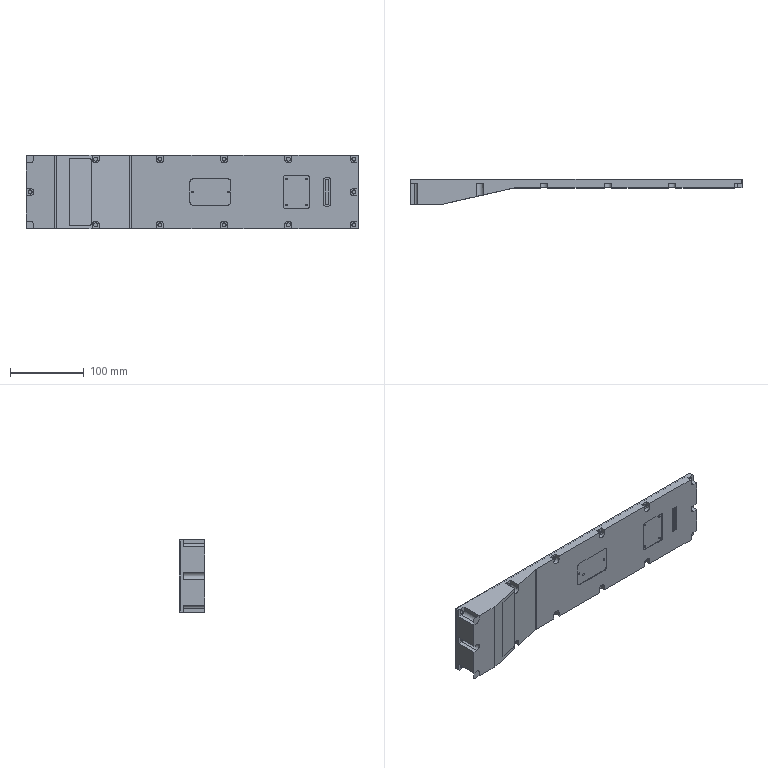NC program | Mastercam | posted with a generic post | part box 450 x 35 x 100 mm
Lines 36 to 1467 of 140701:
(12 FEM |TOOL - 12|DIA. OFF. - 12|LEN. - 12|TOOL DIA. - 12.)
N140 T12 M6
N142 G0 G54 G90 X-233.997 Y-60.496 C0. B0. S7000 M3
N144 G43 H12 Z50.
N146 Z3.
N148 G1 Z-18.575 F600.
N150 X-234.4 Y-59.449 Z-18.7 F4000.
N152 G3 X-235.01 Y-58.51 Z-18.825 I-2.52 J-.971
N154 G1 X-235.205 Y-58.247
N156 X-235.623 Y-57.657
N158 X-235.863 Y-57.277
N160 X-236.1 Y-56.858
N162 X-236.324 Y-56.407
N164 X-236.529 Y-55.928
N166 X-236.708 Y-55.428
N168 X-236.848 Y-54.949
N170 X-236.954 Y-54.508
N172 X-237.033 Y-54.1
N174 X-237.14 Y-53.384
N176 X-237.205 Y-52.737
N178 X-237.245 Y-52.143
N180 X-237.27 Y-51.587
N182 X-237.284 Y-51.058
N184 X-237.293 Y-50.55
N186 X-237.296 Y-50.055
N188 X-237.297 Y-49.569
N190 X-237.296 Y-49.091
N192 X-237.294 Y-48.616
N194 X-237.291 Y-48.145
N196 X-237.287 Y-47.675
N198 X-237.283 Y-47.206
N200 X-237.279 Y-46.738
N202 X-237.275 Y-46.27
N204 X-237.271 Y-45.802
N206 X-237.266 Y-45.334
N208 X-237.262 Y-44.866
N210 X-237.258 Y-44.399
N212 X-237.253 Y-43.931
N214 X-237.249 Y-43.463
N216 X-237.245 Y-42.995
N218 X-237.24 Y-42.526
N220 X-237.236 Y-42.058
N222 X-237.231 Y-41.59
N224 X-237.227 Y-41.121
N226 X-237.222 Y-40.652
N228 X-237.218 Y-40.184
N230 X-237.213 Y-39.715
N232 X-237.209 Y-39.246
N234 X-237.205 Y-38.777
N236 X-237.2 Y-38.307
N238 X-237.196 Y-37.838
N240 X-237.191 Y-37.369
N242 X-237.187 Y-36.899
N244 X-237.182 Y-36.429
N246 X-237.178 Y-35.96
N248 X-237.173 Y-35.49
N250 X-237.169 Y-35.02
N252 X-237.165 Y-34.55
N254 X-237.16 Y-34.08
N256 X-237.156 Y-33.609
N258 X-237.151 Y-33.139
N260 X-237.147 Y-32.669
N262 X-237.142 Y-32.198
N264 X-237.138 Y-31.728
N266 X-237.133 Y-31.257
N268 X-237.129 Y-30.787
N270 X-237.124 Y-30.316
N272 X-237.12 Y-29.845
N274 X-237.116 Y-29.374
N276 X-237.111 Y-28.903
N278 X-237.107 Y-28.432
N280 X-237.102 Y-27.961
N282 X-237.098 Y-27.49
N284 X-237.093 Y-27.018
N286 X-237.089 Y-26.547
N288 X-237.084 Y-26.075
N290 X-237.08 Y-25.604
N292 X-237.075 Y-25.132
N294 X-237.071 Y-24.661
N296 X-237.066 Y-24.189
N298 X-237.062 Y-23.717
N300 X-237.058 Y-23.246
N302 X-237.053 Y-22.774
N304 X-237.049 Y-22.302
N306 X-237.044 Y-21.83
N308 X-237.04 Y-21.358
N310 X-237.035 Y-20.886
N312 X-237.031 Y-20.414
N314 X-237.026 Y-19.941
N316 X-237.022 Y-19.469
N318 X-237.017 Y-18.997
N320 X-237.013 Y-18.524
N322 X-237.008 Y-18.052
N324 X-237.004 Y-17.579
N326 X-236.999 Y-17.107
N328 X-236.995 Y-16.634
N330 X-236.99 Y-16.162
N332 X-236.986 Y-15.689
N334 X-236.982 Y-15.216
N336 X-236.977 Y-14.744
N338 X-236.973 Y-14.271
N340 X-236.968 Y-13.798
N342 X-236.964 Y-13.325
N344 X-236.959 Y-12.852
N346 X-236.955 Y-12.379
N348 X-236.95 Y-11.906
N350 X-236.946 Y-11.433
N352 X-236.941 Y-10.96
N354 X-236.937 Y-10.486
N356 X-236.932 Y-10.013
N358 X-236.928 Y-9.54
N360 X-236.923 Y-9.067
N362 X-236.919 Y-8.593
N364 X-236.914 Y-8.12
N366 X-236.91 Y-7.646
N368 X-236.905 Y-7.173
N370 X-236.901 Y-6.699
N372 X-236.896 Y-6.226
N374 X-236.892 Y-5.752
N376 X-236.887 Y-5.279
N378 X-236.883 Y-4.805
N380 X-236.878 Y-4.331
N382 X-236.874 Y-3.857
N384 X-236.869 Y-3.384
N386 X-236.865 Y-2.91
N388 X-236.861 Y-2.436
N390 X-236.856 Y-1.962
N392 X-236.852 Y-1.488
N394 X-236.847 Y-1.014
N396 X-236.843 Y-.54
N398 X-236.838 Y-.066
N400 X-236.834 Y.408
N402 X-236.829 Y.882
N404 X-236.825 Y1.356
N406 X-236.82 Y1.831
N408 X-236.816 Y2.305
N410 X-236.811 Y2.779
N412 X-236.807 Y3.253
N414 X-236.802 Y3.728
N416 X-236.798 Y4.202
N418 X-236.793 Y4.676
N420 X-236.789 Y5.151
N422 X-236.784 Y5.625
N424 X-236.78 Y6.1
N426 X-236.775 Y6.574
N428 X-236.771 Y7.049
N430 X-236.766 Y7.523
N432 X-236.762 Y7.998
N434 X-236.757 Y8.473
N436 X-236.753 Y8.947
N438 X-236.748 Y9.422
N440 X-236.744 Y9.897
N442 X-236.739 Y10.371
N444 X-236.735 Y10.846
N446 X-236.73 Y11.321
N448 X-236.726 Y11.796
N450 X-236.721 Y12.271
N452 X-236.717 Y12.745
N454 X-236.712 Y13.22
N456 X-236.708 Y13.695
N458 X-236.703 Y14.17
N460 X-236.699 Y14.645
N462 X-236.694 Y15.12
N464 X-236.69 Y15.595
N466 X-236.685 Y16.07
N468 X-236.681 Y16.546
N470 X-236.676 Y17.021
N472 X-236.672 Y17.496
N474 X-236.667 Y17.971
N476 X-236.663 Y18.446
N478 X-236.658 Y18.921
N480 X-236.654 Y19.397
N482 X-236.649 Y19.872
N484 X-236.645 Y20.347
N486 X-236.64 Y20.823
N488 X-236.636 Y21.298
N490 X-236.631 Y21.773
N492 X-236.627 Y22.249
N494 X-236.622 Y22.724
N496 X-236.618 Y23.2
N498 X-236.613 Y23.675
N500 X-236.609 Y24.15
N502 X-236.604 Y24.626
N504 X-236.6 Y25.102
N506 X-236.595 Y25.577
N508 X-236.591 Y26.053
N510 X-236.586 Y26.528
N512 X-236.582 Y27.004
N514 X-236.577 Y27.48
N516 X-236.573 Y27.955
N518 X-236.568 Y28.431
N520 X-236.564 Y28.907
N522 X-236.559 Y29.382
N524 X-236.555 Y29.858
N526 X-236.55 Y30.334
N528 X-236.546 Y30.81
N530 X-236.541 Y31.286
N532 X-236.537 Y31.761
N534 X-236.532 Y32.237
N536 X-236.528 Y32.714
N538 X-236.524 Y33.191
N540 X-236.521 Y33.669
N542 X-236.518 Y34.148
N544 X-236.516 Y34.627
N546 X-236.513 Y35.107
N548 X-236.512 Y35.587
N550 X-236.51 Y36.068
N552 X-236.509 Y36.549
N554 X-236.508 Y37.03
N556 X-236.507 Y37.511
N558 X-236.506 Y37.993
N560 X-236.505 Y38.475
N562 X-236.504 Y38.957
N564 Y39.439
N566 X-236.503 Y39.921
N568 Y40.403
N570 X-236.502 Y40.885
N572 Y41.368
N574 Y41.85
N576 Y42.332
N578 X-236.501 Y42.815
N580 Y43.298
N582 Y43.78
N584 Y44.263
N586 Y44.745
N588 Y45.228
N590 Y45.711
N592 X-236.5 Y46.193
N594 Y46.676
N596 Y47.159
N598 Y47.642
N600 Y48.124
N602 Y48.607
N604 Y49.09
N606 X-236.499 Y49.611
N608 X-236.485 Y50.23
N610 X-236.44 Y50.918
N612 X-236.401 Y51.288
N614 X-236.347 Y51.666
N616 X-236.277 Y52.051
N618 X-236.19 Y52.44
N620 X-236.085 Y52.831
N622 X-235.96 Y53.221
N624 X-235.816 Y53.607
N626 X-235.651 Y53.989
N628 X-235.466 Y54.362
N630 X-235.26 Y54.727
N632 X-235.034 Y55.079
N634 X-234.788 Y55.418
N636 X-234.524 Y55.743
N638 X-234.245 Y56.051
N640 X-233.952 Y56.343
N642 X-233.649 Y56.618
N644 X-233.337 Y56.875
N646 X-233.018 Y57.116
N648 X-232.694 Y57.34
N650 X-232.366 Y57.548
N652 X-232.036 Y57.741
N654 X-231.705 Y57.919
N656 X-231.056 Y58.23
N658 X-230.41 Y58.496
N660 X-229.773 Y58.721
N662 X-229.146 Y58.912
N664 X-228.53 Y59.074
N666 X-227.927 Y59.211
N668 X-227.336 Y59.327
N670 X-226.756 Y59.425
N672 X-226.187 Y59.508
N674 X-225.627 Y59.579
N676 X-225.077 Y59.639
N678 X-224.535 Y59.691
N680 X-224.001 Y59.734
N682 X-223.473 Y59.772
N684 X-222.95 Y59.804
N686 X-222.433 Y59.831
N688 X-221.92 Y59.855
N690 X-221.411 Y59.875
N692 X-220.906 Y59.892
N694 X-220.403 Y59.907
N696 X-219.903 Y59.92
N698 X-219.406 Y59.931
N700 X-218.91 Y59.94
N702 X-218.416 Y59.949
N704 X-217.924 Y59.956
N706 X-217.433 Y59.962
N708 X-216.942 Y59.967
N710 X-216.453 Y59.971
N712 X-215.965 Y59.975
N714 X-215.478 Y59.979
N716 X-214.991 Y59.982
N718 X-214.505 Y59.984
N720 X-214.019 Y59.986
N722 X-213.533 Y59.988
N724 X-213.048 Y59.99
N726 X-212.563 Y59.991
N728 X-212.079 Y59.992
N730 X-211.595 Y59.993
N732 X-211.111 Y59.994
N734 X-210.627 Y59.995
N736 X-210.143 Y59.996
N738 X-209.659
N740 X-209.176 Y59.997
N742 X-208.692
N744 X-208.209 Y59.998
N746 X-207.726
N748 X-207.243
N750 X-206.759
N752 X-206.276 Y59.999
N754 X-205.793
N756 X-205.31
N758 X-204.827
N760 X-204.344
N762 X-203.861
N764 X-203.378
N766 X-202.895 Y60.
N768 X-202.412
N770 X-201.93
N772 X-201.447
N774 X-200.964
N776 X-200.481
N778 X-199.998
N780 X-199.515
N782 X-199.032
N784 X-198.55
N786 X-198.067
N788 X-197.584
N790 X-197.101
N792 X-196.618
N794 X-196.135
N796 X-195.653
N798 X-195.17
N800 X-194.687
N802 X-194.204
N804 X-193.721
N806 X-193.238
N808 X-192.756
N810 X-192.273
N812 X-191.79
N814 X-191.307
N816 X-190.824
N818 X-190.342
N820 X-189.859
N822 X-189.376
N824 X-188.893
N826 X-188.41
N828 X-187.927
N830 X-187.445
N832 X-186.962
N834 X-186.479
N836 X-185.996
N838 X-185.513
N840 X-185.031
N842 X-184.548
N844 X-184.065
N846 X-183.582
N848 X-183.099
N850 X-182.616
N852 X-182.134
N854 X-181.651
N856 X-181.168
N858 X-180.685
N860 X-180.202
N862 X-179.72
N864 X-179.237
N866 X-178.754
N868 X-178.271
N870 X-177.788
N872 X-177.306
N874 X-176.823
N876 X-176.34
N878 X-175.857
N880 X-175.374
N882 X-174.891
N884 X-174.409
N886 X-173.926
N888 X-173.443
N890 X-172.96
N892 X-172.477
N894 X-171.995
N896 X-171.512
N898 X-171.029
N900 X-170.546
N902 X-170.063
N904 X-169.581
N906 X-169.098
N908 X-168.615
N910 X-168.132
N912 X-167.649
N914 X-167.166
N916 X-166.684
N918 X-166.201
N920 X-165.718
N922 X-165.235
N924 X-164.752
N926 X-164.27
N928 X-163.787
N930 X-163.304
N932 X-162.821
N934 X-162.338
N936 X-161.856
N938 X-161.373
N940 X-160.89
N942 X-160.407
N944 X-159.924
N946 X-159.441
N948 X-158.959
N950 X-158.476
N952 X-157.993
N954 X-157.51
N956 X-157.027
N958 X-156.545
N960 X-156.062
N962 X-155.579
N964 X-155.096
N966 X-154.613
N968 X-154.131
N970 X-153.648
N972 X-153.165
N974 X-152.682
N976 X-152.199
N978 X-151.716
N980 X-151.234
N982 X-150.751
N984 X-150.268
N986 X-149.785
N988 X-149.302
N990 X-148.82
N992 X-148.337
N994 X-147.854
N996 X-147.371
N998 X-146.888
N1000 X-146.406
N1002 X-145.923
N1004 X-145.44
N1006 X-144.957
N1008 X-144.474
N1010 X-143.991
N1012 X-143.509
N1014 X-143.026
N1016 X-142.543
N1018 X-142.06
N1020 X-141.577
N1022 X-141.095
N1024 X-140.612
N1026 X-140.129
N1028 X-139.646
N1030 X-139.163
N1032 X-138.681
N1034 X-138.198
N1036 X-137.715
N1038 X-137.232
N1040 X-136.749
N1042 X-136.266
N1044 X-135.784
N1046 X-135.301
N1048 X-134.818
N1050 X-134.335
N1052 X-133.852
N1054 X-133.37
N1056 X-132.887
N1058 X-132.404
N1060 X-131.921
N1062 X-131.438
N1064 X-130.956
N1066 X-130.473
N1068 X-129.99
N1070 X-129.507
N1072 X-129.024
N1074 X-128.542
N1076 X-128.059
N1078 X-127.576
N1080 X-127.093
N1082 X-126.61
N1084 X-126.127
N1086 X-125.645
N1088 X-125.162
N1090 X-124.679
N1092 X-124.196
N1094 X-123.713
N1096 X-123.231
N1098 X-122.748
N1100 X-122.265
N1102 X-121.782
N1104 X-121.299
N1106 X-120.817
N1108 X-120.334
N1110 X-119.851
N1112 X-119.368
N1114 X-118.885
N1116 X-118.402
N1118 X-117.92
N1120 X-117.437
N1122 X-116.954
N1124 X-116.471
N1126 X-115.988
N1128 X-115.506
N1130 X-115.023
N1132 X-114.54
N1134 X-114.057
N1136 X-113.574
N1138 X-113.092
N1140 X-112.609
N1142 X-112.126
N1144 X-111.643
N1146 X-111.16
N1148 X-110.677
N1150 X-110.195
N1152 X-109.712
N1154 X-109.229
N1156 X-108.746
N1158 X-108.263
N1160 X-107.781
N1162 X-107.298
N1164 X-106.815
N1166 X-106.332
N1168 X-105.849
N1170 X-105.367
N1172 X-104.884
N1174 X-104.401
N1176 X-103.918
N1178 X-103.435
N1180 X-102.952
N1182 X-102.47
N1184 X-101.987
N1186 X-101.504
N1188 X-101.021
N1190 X-100.538
N1192 X-100.056
N1194 X-99.573
N1196 X-99.09
N1198 X-98.607
N1200 X-98.124
N1202 X-97.642
N1204 X-97.159
N1206 X-96.676
N1208 X-96.193
N1210 X-95.71
N1212 X-95.227
N1214 X-94.745
N1216 X-94.262
N1218 X-93.779
N1220 X-93.296
N1222 X-92.813
N1224 X-92.331
N1226 X-91.848
N1228 X-91.365
N1230 X-90.882
N1232 X-90.399
N1234 X-89.917
N1236 X-89.434
N1238 X-88.951
N1240 X-88.468
N1242 X-87.985
N1244 X-87.502
N1246 X-87.02
N1248 X-86.537
N1250 X-86.054
N1252 X-85.571
N1254 X-85.088
N1256 X-84.606
N1258 X-84.123
N1260 X-83.64
N1262 X-83.157
N1264 X-82.674
N1266 X-82.192
N1268 X-81.709
N1270 X-81.226
N1272 X-80.743
N1274 X-80.26
N1276 X-79.777
N1278 X-79.295
N1280 X-78.812
N1282 X-78.329
N1284 X-77.846
N1286 X-77.363
N1288 X-76.881
N1290 X-76.398
N1292 X-75.915
N1294 X-75.432
N1296 X-74.949
N1298 X-74.467
N1300 X-73.984
N1302 X-73.501
N1304 X-73.018
N1306 X-72.535
N1308 X-72.052
N1310 X-71.57
N1312 X-71.087
N1314 X-70.604
N1316 X-70.121
N1318 X-69.638
N1320 X-69.156
N1322 X-68.673
N1324 X-68.19
N1326 X-67.707
N1328 X-67.224
N1330 X-66.742
N1332 X-66.259
N1334 X-65.776
N1336 X-65.293
N1338 X-64.81
N1340 X-64.327
N1342 X-63.845
N1344 X-63.362
N1346 X-62.879
N1348 X-62.396
N1350 X-61.913
N1352 X-61.431
N1354 X-60.948
N1356 X-60.465
N1358 X-59.982
N1360 X-59.499
N1362 X-59.017
N1364 X-58.534
N1366 X-58.051
N1368 X-57.568
N1370 X-57.085
N1372 X-56.602
N1374 X-56.12
N1376 X-55.637
N1378 X-55.154
N1380 X-54.671
N1382 X-54.188
N1384 X-53.706
N1386 X-53.223
N1388 X-52.74
N1390 X-52.257
N1392 X-51.774
N1394 X-51.292
N1396 X-50.809
N1398 X-50.326
N1400 X-49.843
N1402 X-49.36
N1404 X-48.877
N1406 X-48.395
N1408 X-47.912
N1410 X-47.429
N1412 X-46.946
N1414 X-46.463
N1416 X-45.981
N1418 X-45.498
N1420 X-45.015
N1422 X-44.532
N1424 X-44.049
N1426 X-43.567
N1428 X-43.084
N1430 X-42.601
N1432 X-42.118
N1434 X-41.635
N1436 X-41.152
N1438 X-40.67
N1440 X-40.187
N1442 X-39.704
N1444 X-39.221
N1446 X-38.738
N1448 X-38.256
N1450 X-37.773
N1452 X-37.29
N1454 X-36.807
N1456 X-36.324
N1458 X-35.842
N1460 X-35.359
N1462 X-34.876
N1464 X-34.393
N1466 X-33.91
N1468 X-33.427
N1470 X-32.945
N1472 X-32.462
N1474 X-31.979
N1476 X-31.496
N1478 X-31.013
N1480 X-30.531
N1482 X-30.048
N1484 X-29.565
N1486 X-29.082
N1488 X-28.599
N1490 X-28.117
N1492 X-27.634
N1494 X-27.151
N1496 X-26.668
N1498 X-26.185
N1500 X-25.702
N1502 X-25.22
N1504 X-24.737
N1506 X-24.254
N1508 X-23.771
N1510 X-23.288
N1512 X-22.806
N1514 X-22.323
N1516 X-21.84
N1518 X-21.357
N1520 X-20.874
N1522 X-20.392
N1524 X-19.909
N1526 X-19.426
N1528 X-18.943
N1530 X-18.46
N1532 X-17.977
N1534 X-17.495
N1536 X-17.012
N1538 X-16.529
N1540 X-16.046
N1542 X-15.563
N1544 X-15.081
N1546 X-14.598
N1548 X-14.115
N1550 X-13.632
N1552 X-13.149
N1554 X-12.667
N1556 X-12.184
N1558 X-11.701
N1560 X-11.218
N1562 X-10.735
N1564 X-10.252
N1566 X-9.77
N1568 X-9.287
N1570 X-8.804
N1572 X-8.321
N1574 X-7.838
N1576 X-7.356
N1578 X-6.873
N1580 X-6.39
N1582 X-5.907
N1584 X-5.424
N1586 X-4.942
N1588 X-4.459
N1590 X-3.976
N1592 X-3.493
N1594 X-3.01
N1596 X-2.527
N1598 X-2.045
N1600 X-1.562
N1602 X-1.079
N1604 X-.596
N1606 X-.113
N1608 X.369
N1610 X.852
N1612 X1.335
N1614 X1.818
N1616 X2.301
N1618 X2.783
N1620 X3.266
N1622 X3.749
N1624 X4.232
N1626 X4.715
N1628 X5.198
N1630 X5.68
N1632 X6.163
N1634 X6.646
N1636 X7.129
N1638 X7.612
N1640 X8.094
N1642 X8.577
N1644 X9.06
N1646 X9.543
N1648 X10.026
N1650 X10.508
N1652 X10.991
N1654 X11.474
N1656 X11.957
N1658 X12.44
N1660 X12.923
N1662 X13.405
N1664 X13.888
N1666 X14.371
N1668 X14.854
N1670 X15.337
N1672 X15.819
N1674 X16.302
N1676 X16.785
N1678 X17.268
N1680 X17.751
N1682 X18.233
N1684 X18.716
N1686 X19.199
N1688 X19.682
N1690 X20.165
N1692 X20.648
N1694 X21.13
N1696 X21.613
N1698 X22.096
N1700 X22.579
N1702 X23.062
N1704 X23.544
N1706 X24.027
N1708 X24.51
N1710 X24.993
N1712 X25.476
N1714 X25.958
N1716 X26.441
N1718 X26.924
N1720 X27.407
N1722 X27.89
N1724 X28.373
N1726 X28.855
N1728 X29.338
N1730 X29.821
N1732 X30.304
N1734 X30.787
N1736 X31.269
N1738 X31.752
N1740 X32.235
N1742 X32.718
N1744 X33.201
N1746 X33.683
N1748 X34.166
N1750 X34.649
N1752 X35.132
N1754 X35.615
N1756 X36.098
N1758 X36.58
N1760 X37.063
N1762 X37.546
N1764 X38.029
N1766 X38.512
N1768 X38.994
N1770 X39.477
N1772 X39.96
N1774 X40.443
N1776 X40.926
N1778 X41.408
N1780 X41.891
N1782 X42.374
N1784 X42.857
N1786 X43.34
N1788 X43.823
N1790 X44.305
N1792 X44.788
N1794 X45.271
N1796 X45.754
N1798 X46.237
N1800 X46.719
N1802 X47.202
N1804 X47.685
N1806 X48.168
N1808 X48.651
N1810 X49.133
N1812 X49.616
N1814 X50.099
N1816 X50.582
N1818 X51.065
N1820 X51.548
N1822 X52.03
N1824 X52.513
N1826 X52.996
N1828 X53.479
N1830 X53.962
N1832 X54.444
N1834 X54.927
N1836 X55.41
N1838 X55.893
N1840 X56.376
N1842 X56.858
N1844 X57.341
N1846 X57.824
N1848 X58.307
N1850 X58.79
N1852 X59.273
N1854 X59.755
N1856 X60.238
N1858 X60.721
N1860 X61.204
N1862 X61.687
N1864 X62.169
N1866 X62.652
N1868 X63.135
N1870 X63.618
N1872 X64.101
N1874 X64.583
N1876 X65.066
N1878 X65.549
N1880 X66.032
N1882 X66.515
N1884 X66.998
N1886 X67.48
N1888 X67.963
N1890 X68.446
N1892 X68.929
N1894 X69.412
N1896 X69.894
N1898 X70.377
N1900 X70.86
N1902 X71.343
N1904 X71.826
N1906 X72.308
N1908 X72.791
N1910 X73.274
N1912 X73.757
N1914 X74.24
N1916 X74.723
N1918 X75.205
N1920 X75.688
N1922 X76.171
N1924 X76.654
N1926 X77.137
N1928 X77.619
N1930 X78.102
N1932 X78.585
N1934 X79.068
N1936 X79.551
N1938 X80.033
N1940 X80.516
N1942 X80.999
N1944 X81.482
N1946 X81.965
N1948 X82.448
N1950 X82.93
N1952 X83.413
N1954 X83.896
N1956 X84.379
N1958 X84.862
N1960 X85.344
N1962 X85.827
N1964 X86.31
N1966 X86.793
N1968 X87.276
N1970 X87.758
N1972 X88.241
N1974 X88.724
N1976 X89.207
N1978 X89.69
N1980 X90.173
N1982 X90.655
N1984 X91.138
N1986 X91.621
N1988 X92.104
N1990 X92.587
N1992 X93.069
N1994 X93.552
N1996 X94.035
N1998 X94.518
N2000 X95.001
N2002 X95.483
N2004 X95.966
N2006 X96.449
N2008 X96.932
N2010 X97.415
N2012 X97.898
N2014 X98.38
N2016 X98.863
N2018 X99.346
N2020 X99.829
N2022 X100.312
N2024 X100.794
N2026 X101.277
N2028 X101.76
N2030 X102.243
N2032 X102.726
N2034 X103.208
N2036 X103.691
N2038 X104.174
N2040 X104.657
N2042 X105.14
N2044 X105.623
N2046 X106.105
N2048 X106.588
N2050 X107.071
N2052 X107.554
N2054 X108.037
N2056 X108.519
N2058 X109.002
N2060 X109.485
N2062 X109.968
N2064 X110.451
N2066 X110.933
N2068 X111.416
N2070 X111.899
N2072 X112.382
N2074 X112.865
N2076 X113.348
N2078 X113.83
N2080 X114.313
N2082 X114.796
N2084 X115.279
N2086 X115.762
N2088 X116.244
N2090 X116.727
N2092 X117.21
N2094 X117.693
N2096 X118.176
N2098 X118.658
N2100 X119.141
N2102 X119.624
N2104 X120.107
N2106 X120.59
N2108 X121.073
N2110 X121.555
N2112 X122.038
N2114 X122.521
N2116 X123.004
N2118 X123.487
N2120 X123.969
N2122 X124.452
N2124 X124.935
N2126 X125.418
N2128 X125.901
N2130 X126.383
N2132 X126.866
N2134 X127.349
N2136 X127.832
N2138 X128.315
N2140 X128.798
N2142 X129.28
N2144 X129.763
N2146 X130.246
N2148 X130.729
N2150 X131.212
N2152 X131.694
N2154 X132.177
N2156 X132.66
N2158 X133.143
N2160 X133.626
N2162 X134.108
N2164 X134.591
N2166 X135.074
N2168 X135.557
N2170 X136.04
N2172 X136.523
N2174 X137.005
N2176 X137.488
N2178 X137.971
N2180 X138.454
N2182 X138.937
N2184 X139.419
N2186 X139.902
N2188 X140.385
N2190 X140.868
N2192 X141.351
N2194 X141.833
N2196 X142.316
N2198 X142.799
N2200 X143.282
N2202 X143.765
N2204 X144.247
N2206 X144.73
N2208 X145.213
N2210 X145.696
N2212 X146.179
N2214 X146.662
N2216 X147.144
N2218 X147.627
N2220 X148.11
N2222 X148.593
N2224 X149.076
N2226 X149.558
N2228 X150.041
N2230 X150.524
N2232 X151.007
N2234 X151.49
N2236 X151.972
N2238 X152.455
N2240 X152.938
N2242 X153.421
N2244 X153.904
N2246 X154.387
N2248 X154.869
N2250 X155.352
N2252 X155.835
N2254 X156.318
N2256 X156.801
N2258 X157.283
N2260 X157.766
N2262 X158.249
N2264 X158.732
N2266 X159.215
N2268 X159.697
N2270 X160.18
N2272 X160.663
N2274 X161.146
N2276 X161.629
N2278 X162.112
N2280 X162.594
N2282 X163.077
N2284 X163.56
N2286 X164.043
N2288 X164.526
N2290 X165.008
N2292 X165.491
N2294 X165.974
N2296 X166.457
N2298 X166.94
N2300 X167.422
N2302 X167.905
N2304 X168.388
N2306 X168.871
N2308 X169.354
N2310 X169.837
N2312 X170.319
N2314 X170.802
N2316 X171.285
N2318 X171.768
N2320 X172.251
N2322 X172.733
N2324 X173.216
N2326 X173.699
N2328 X174.182
N2330 X174.665
N2332 X175.147
N2334 X175.63
N2336 X176.113
N2338 X176.596
N2340 X177.079
N2342 X177.562
N2344 X178.044
N2346 X178.527
N2348 X179.01
N2350 X179.493
N2352 X179.976
N2354 X180.458
N2356 X180.941
N2358 X181.424
N2360 X181.907
N2362 X182.39
N2364 X182.872
N2366 X183.355
N2368 X183.838
N2370 X184.321
N2372 X184.804
N2374 X185.287
N2376 X185.769
N2378 X186.252
N2380 X186.735
N2382 X187.218
N2384 X187.701
N2386 X188.183
N2388 X188.666
N2390 X189.149
N2392 X189.632
N2394 X190.115
N2396 X190.597
N2398 X191.08
N2400 X191.563
N2402 X192.046
N2404 X192.529
N2406 X193.012
N2408 X193.494
N2410 X193.977
N2412 X194.46
N2414 X194.943
N2416 X195.426
N2418 X195.908
N2420 X196.391
N2422 X196.874
N2424 X197.357
N2426 X197.84
N2428 X198.322
N2430 X198.805
N2432 X199.288
N2434 X199.771
N2436 X200.254
N2438 X200.737
N2440 X201.219
N2442 X201.702
N2444 X202.185
N2446 X202.668
N2448 X203.151
N2450 X203.633
N2452 X204.116
N2454 X204.599
N2456 X205.082
N2458 X205.565
N2460 X206.047
N2462 X206.53
N2464 X207.013
N2466 X207.496
N2468 X207.979
N2470 X208.462
N2472 X208.944
N2474 X209.427
N2476 X209.91
N2478 X210.393
N2480 X210.876
N2482 X211.358
N2484 X211.841
N2486 X212.324
N2488 X212.807
N2490 X213.29
N2492 X213.772
N2494 X214.255
N2496 X214.738
N2498 X215.221
N2500 X215.704
N2502 X216.187
N2504 X216.669
N2506 X217.152
N2508 X217.635
N2510 X218.118
N2512 X218.601
N2514 X219.083
N2516 X219.566
N2518 X220.049
N2520 X220.532
N2522 X221.015
N2524 X221.497
N2526 X221.98
N2528 X222.463
N2530 X222.946
N2532 X223.429
N2534 X223.912
N2536 X224.394
N2538 X224.877
N2540 X225.36
N2542 X225.849
N2544 X226.425 Y59.994
N2546 X227.084 Y59.966
N2548 X227.798 Y59.899
N2550 X228.177 Y59.845
N2552 X228.562 Y59.775
N2554 X228.952 Y59.687
N2556 X229.342 Y59.582
N2558 X229.732 Y59.457
N2560 X230.119 Y59.312
N2562 X230.5 Y59.146
N2564 X230.873 Y58.96
N2566 X231.237 Y58.754
N2568 X231.589 Y58.527
N2570 X231.928 Y58.28
N2572 X232.252 Y58.016
N2574 X232.56 Y57.736
N2576 X232.851 Y57.444
N2578 X233.125 Y57.14
N2580 X233.382 Y56.828
N2582 X233.622 Y56.509
N2584 X233.846 Y56.184
N2586 X234.054 Y55.856
N2588 X234.246 Y55.526
N2590 X234.424 Y55.195
N2592 X234.734 Y54.546
N2594 X234.999 Y53.901
N2596 X235.224 Y53.264
N2598 X235.415 Y52.637
N2600 X235.576 Y52.021
N2602 X235.712 Y51.418
N2604 X235.828 Y50.827
N2606 X235.926 Y50.247
N2608 X236.009 Y49.678
N2610 X236.08 Y49.119
N2612 X236.14 Y48.569
N2614 X236.191 Y48.027
N2616 X236.235 Y47.493
N2618 X236.272 Y46.965
N2620 X236.304 Y46.443
N2622 X236.332 Y45.925
N2624 X236.355 Y45.413
N2626 X236.375 Y44.904
N2628 X236.392 Y44.398
N2630 X236.407 Y43.896
N2632 X236.42 Y43.396
N2634 X236.431 Y42.898
N2636 X236.441 Y42.403
N2638 X236.449 Y41.909
N2640 X236.456 Y41.416
N2642 X236.462 Y40.925
N2644 X236.467 Y40.435
N2646 X236.471 Y39.946
N2648 X236.475 Y39.458
N2650 X236.479 Y38.971
N2652 X236.482 Y38.484
N2654 X236.484 Y37.997
N2656 X236.486 Y37.512
N2658 X236.488 Y37.026
N2660 X236.49 Y36.541
N2662 X236.491 Y36.056
N2664 X236.492 Y35.572
N2666 X236.493 Y35.088
N2668 X236.494 Y34.603
N2670 X236.495 Y34.12
N2672 X236.496 Y33.636
N2674 Y33.152
N2676 X236.497 Y32.669
N2678 Y32.185
N2680 X236.498 Y31.702
N2682 Y31.219
N2684 Y30.735
N2686 Y30.252
N2688 X236.499 Y29.769
N2690 Y29.286
N2692 Y28.803
N2694 Y28.32
N2696 Y27.837
N2698 Y27.354
N2700 Y26.871
N2702 X236.5 Y26.388
N2704 Y25.905
N2706 Y25.422
N2708 Y24.94
N2710 Y24.457
N2712 Y23.974
N2714 Y23.491
N2716 Y23.008
N2718 Y22.525
N2720 Y22.042
N2722 Y21.56
N2724 Y21.077
N2726 Y20.594
N2728 Y20.111
N2730 Y19.628
N2732 Y19.145
N2734 Y18.663
N2736 Y18.18
N2738 Y17.697
N2740 Y17.214
N2742 Y16.731
N2744 Y16.249
N2746 Y15.766
N2748 Y15.283
N2750 Y14.8
N2752 Y14.317
N2754 Y13.834
N2756 Y13.352
N2758 Y12.869
N2760 Y12.386
N2762 Y11.903
N2764 Y11.42
N2766 Y10.938
N2768 Y10.455
N2770 Y9.972
N2772 Y9.489
N2774 Y9.006
N2776 Y8.523
N2778 Y8.041
N2780 Y7.558
N2782 Y7.075
N2784 Y6.592
N2786 Y6.109
N2788 Y5.627
N2790 Y5.144
N2792 Y4.661
N2794 Y4.178
N2796 Y3.695
N2798 Y3.213
N2800 Y2.73
N2802 Y2.247
N2804 Y1.764
N2806 Y1.281
N2808 Y.798
N2810 Y.316
N2812 Y-.167
N2814 Y-.65
N2816 Y-1.133
N2818 Y-1.616
N2820 Y-2.098
N2822 Y-2.581
N2824 Y-3.064
N2826 Y-3.547
N2828 Y-4.03
N2830 Y-4.512
N2832 Y-4.995
N2834 Y-5.478
N2836 Y-5.961
N2838 Y-6.444
N2840 Y-6.927
N2842 Y-7.409
N2844 Y-7.892
N2846 Y-8.375
N2848 Y-8.858
N2850 Y-9.341
N2852 Y-9.823
N2854 Y-10.306
N2856 Y-10.789
N2858 Y-11.272
N2860 Y-11.755
N2862 Y-12.237
N2864 Y-12.72
N2866 Y-13.203
N2868 Y-13.686
N2870 Y-14.169
N2872 Y-14.652
N2874 Y-15.134
N2876 Y-15.617
N2878 Y-16.1
N2880 Y-16.583
N2882 Y-17.066
N2884 Y-17.548
N2886 Y-18.031
N2888 Y-18.514
N2890 Y-18.997
N2892 Y-19.48
N2894 Y-19.962
N2896 Y-20.445
N2898 Y-20.928
N2900 Y-21.411
N2902 Y-21.894
N2904 Y-22.377
N2906 Y-22.859
N2908 Y-23.342
N2910 Y-23.825
N2912 Y-24.308
N2914 Y-24.791
N2916 Y-25.273
N2918 Y-25.756
N2920 Y-26.239
N2922 Y-26.722
N2924 Y-27.205
N2926 Y-27.687
N2928 Y-28.17
N2930 Y-28.653
N2932 Y-29.136
N2934 Y-29.619
N2936 Y-30.102
N2938 Y-30.584
N2940 Y-31.067
N2942 Y-31.55
N2944 Y-32.033
N2946 Y-32.516
N2948 Y-32.998
N2950 Y-33.481
N2952 Y-33.964
N2954 Y-34.447
N2956 Y-34.93
N2958 Y-35.412
N2960 Y-35.895
N2962 Y-36.378
N2964 Y-36.861
N2966 Y-37.344
N2968 Y-37.827
N2970 Y-38.309
N2972 Y-38.792
N2974 Y-39.275
N2976 Y-39.758
N2978 Y-40.241
N2980 Y-40.723
N2982 Y-41.206
N2984 Y-41.689
N2986 Y-42.172
N2988 Y-42.655
N2990 Y-43.137
N2992 Y-43.62
N2994 Y-44.103
N2996 Y-44.586
N2998 Y-45.069
N3000 Y-45.552